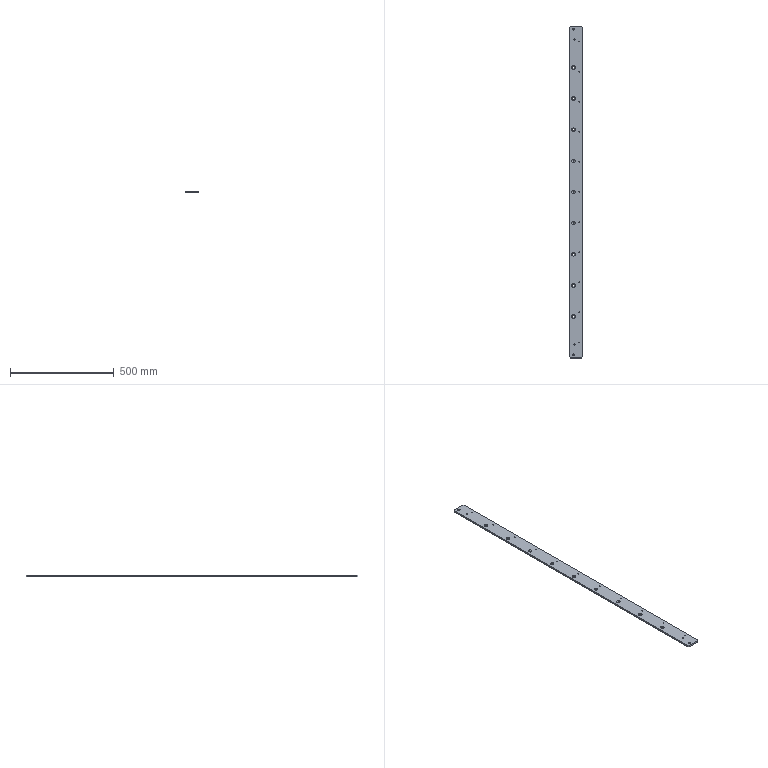Part | NX | features BREP 1 | 1 solid | 76 faces | box 65 x 1600 x 8 mm | volume 820861 mm3 | cylinder 48 | cone 18 | plane 10 | commonest cylinder face diameters 4.2 x22 9 x18 6.8 x4 10 x4